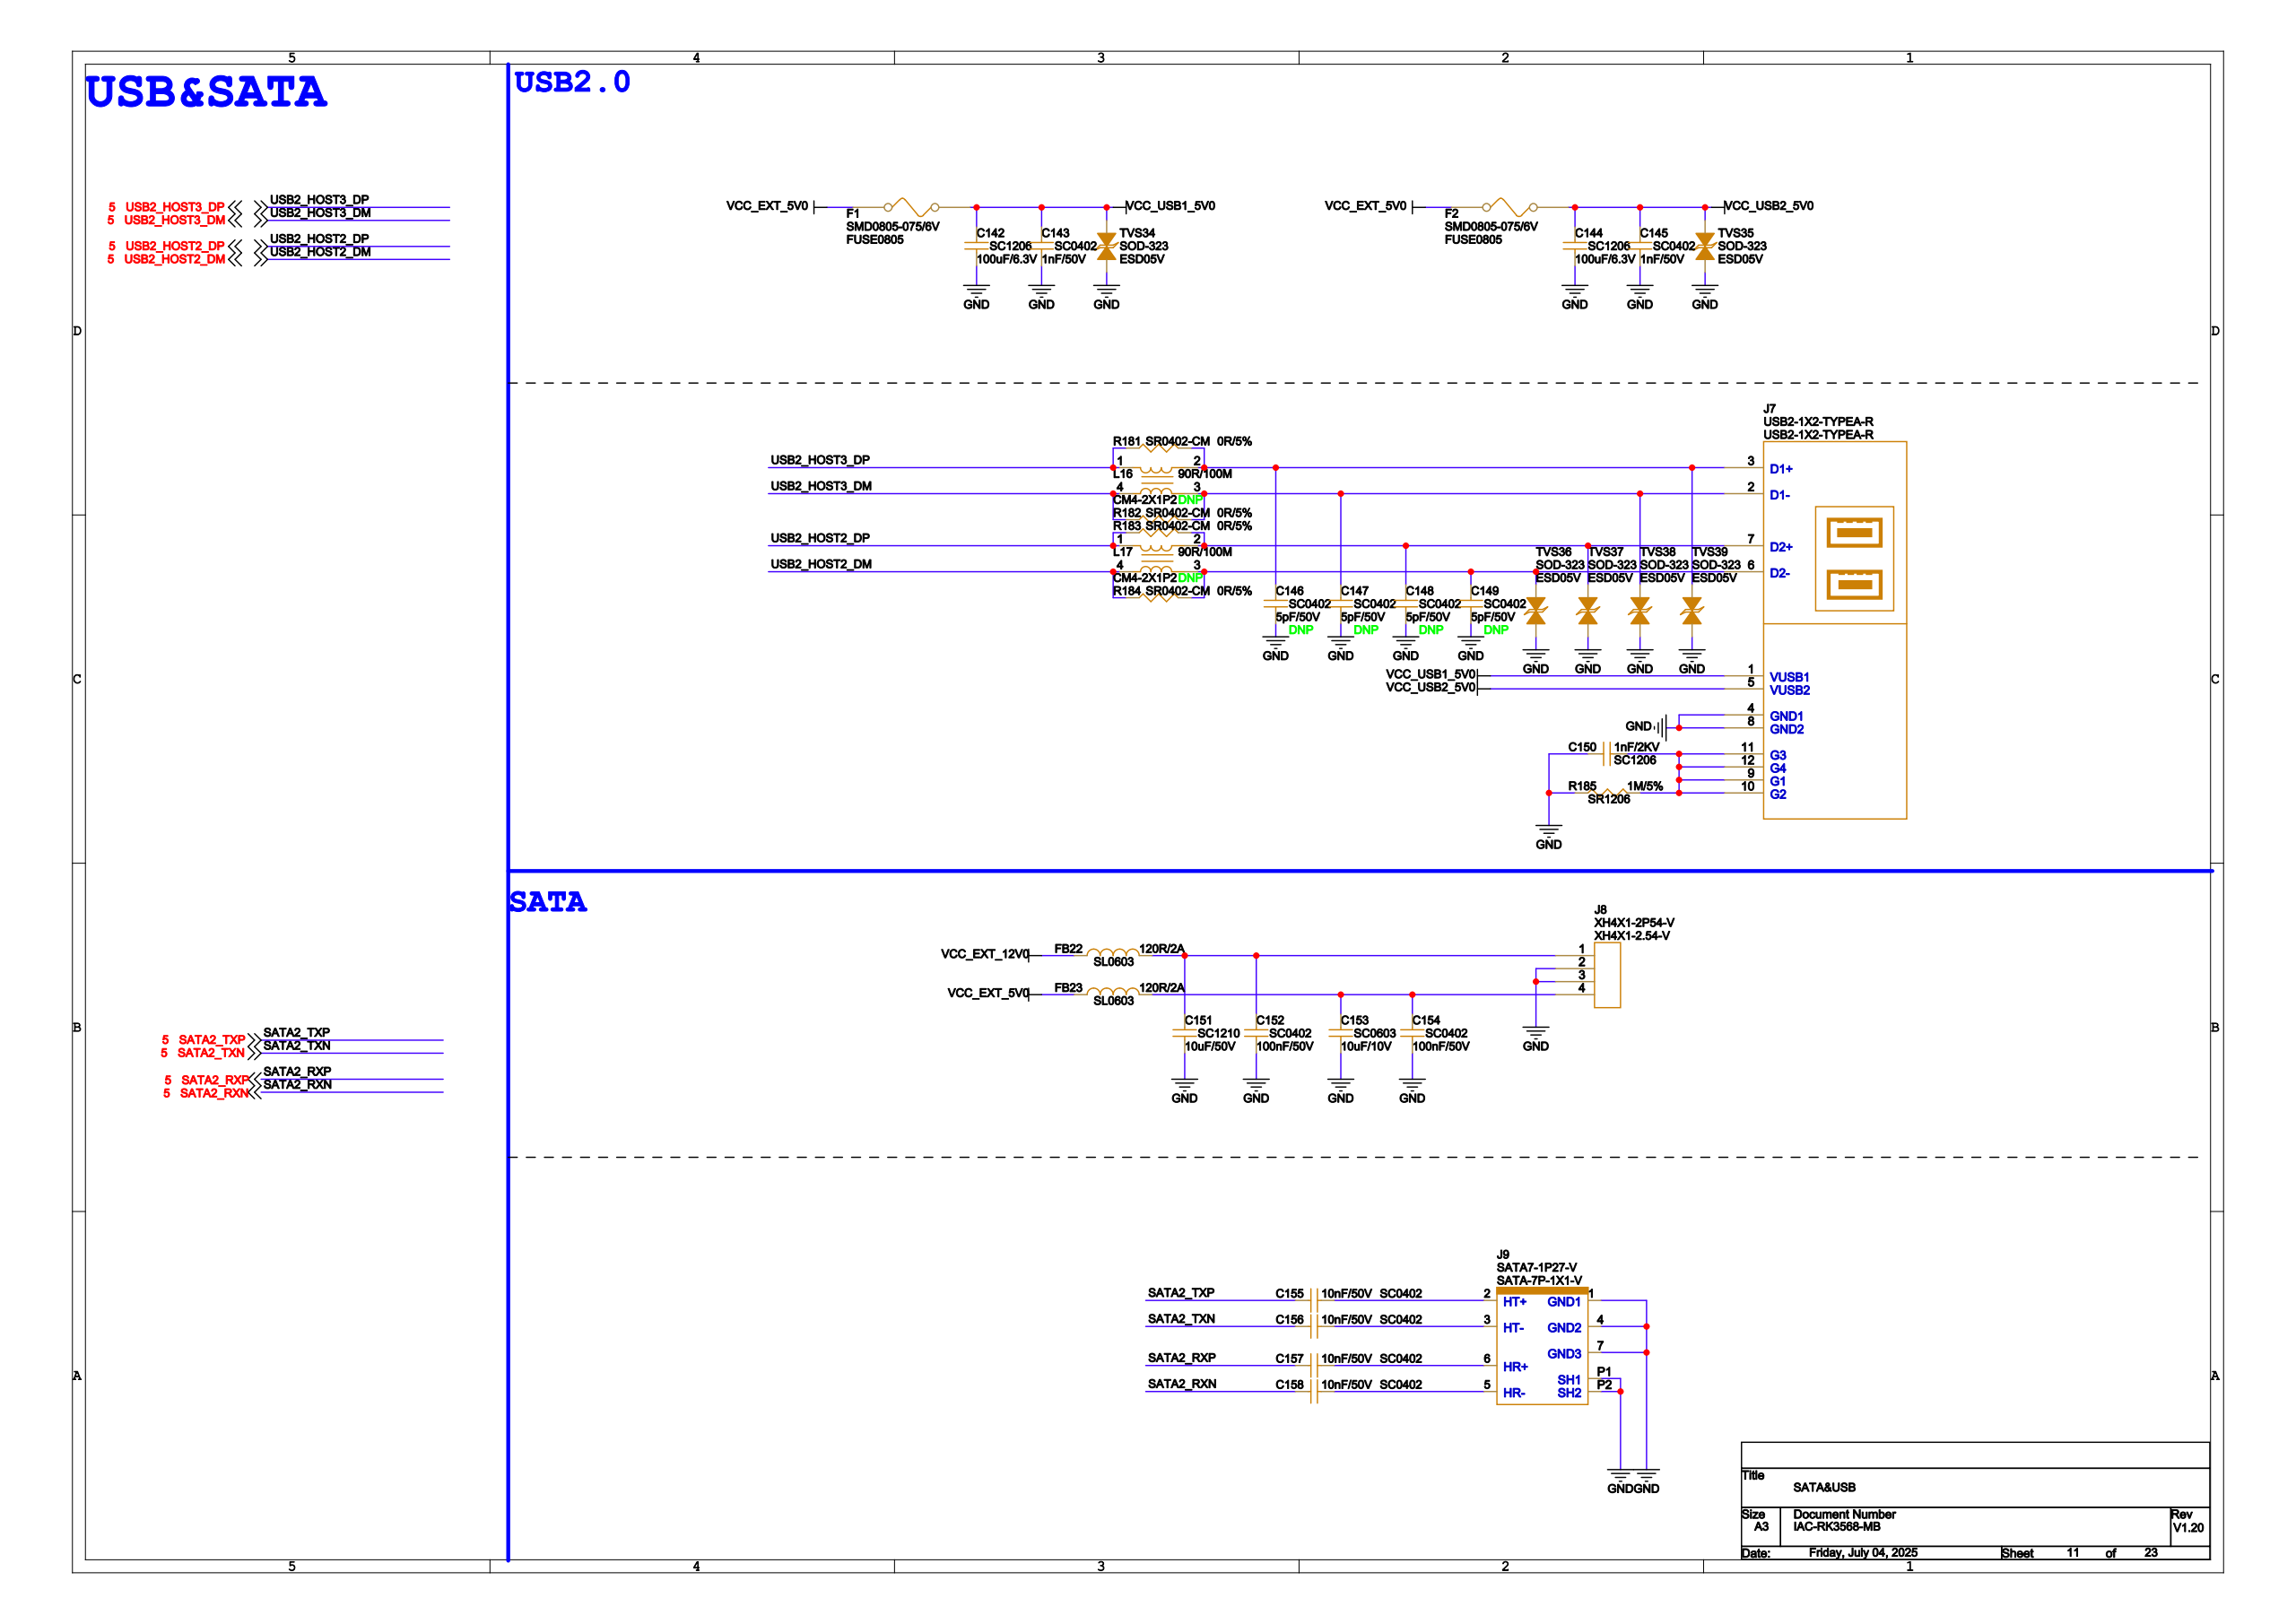Circuit board | Cadence Allegro | 1138 parts | 722 nets | one sheet of the schematic
Parts on this sheet (reference | value | footprint):
C142 | 100uF/6.3V | SC1206
C143 | 1nF/50V | SC0402
C144 | 100uF/6.3V | SC1206
C145 | 1nF/50V | SC0402
C146 | 5pF/50V | SC0402
C147 | 5pF/50V | SC0402
C148 | 5pF/50V | SC0402
C149 | 5pF/50V | SC0402
C150 | 1nF/2KV | SC1206
C151 | 10uF/50V | SC1210
C152 | 100nF/50V | SC0402
C153 | 10uF/10V | SC0603
C154 | 100nF/50V | SC0402
C155 | 10nF/50V | SC0402
C156 | 10nF/50V | SC0402
C157 | 10nF/50V | SC0402
C158 | 10nF/50V | SC0402
F1 | SMD0805-075/6V | FUSE0805
F2 | SMD0805-075/6V | FUSE0805
FB22 | 120R/2A | SL0603
FB23 | 120R/2A | SL0603
J7 | USB2-1X2-TYPEA-R | USB2-1X2-TYPEA-R
J8 | XH4X1-2.54-V | XH4X1-2P54-V
J9 | SATA-7P-1X1-V | SATA7-1P27-V
L16 | 90R/100M | CM4-2X1P2
L17 | 90R/100M | CM4-2X1P2
R181 | 0R/5% | SR0402-CM
R182 | 0R/5% | SR0402-CM
R183 | 0R/5% | SR0402-CM
R184 | 0R/5% | SR0402-CM
R185 | 1M/5% | SR1206
TVS34 | ESD05V | SOD-323
TVS35 | ESD05V | SOD-323
TVS36 | ESD05V | SOD-323
TVS37 | ESD05V | SOD-323
TVS38 | ESD05V | SOD-323
TVS39 | ESD05V | SOD-323
Nets of these parts (net: part-pin ...):
VCC_EXT_5V0: F1-2 F2-2 FB23-1
GND: C142-2 C143-2 C144-2 C145-2 C146-2 C147-2 C148-2 C149-2 C150-1 C151-2 C152-2 C153-2 C154-2 J7-4 J7-8 J8-2 J8-3 J9-1 J9-4 J9-7 J9-P1 J9-P2 R185-1 TVS34-2 TVS35-2 TVS36-1 TVS37-1 TVS38-1 TVS39-1
VCC_USB1_5V0: C142-1 C143-1 F1-1 J7-1 TVS34-1
VCC_USB2_5V0: C144-1 C145-1 F2-1 J7-5 TVS35-1
N3708542: C149-1 J7-6 L17-3 R184-2 TVS36-2
N3708514: C148-1 J7-7 L17-2 R183-2 TVS37-2
N3708486: C147-1 J7-2 L16-3 R182-2 TVS38-2
N3708458: C146-1 J7-3 L16-2 R181-2 TVS39-2
USB2_HOST3_DP: L16-1 R181-1
USB2_HOST3_DM: L16-4 R182-1
USB2_HOST2_DP: L17-1 R183-1
USB2_HOST2_DM: L17-4 R184-1
N4056971: C151-1 C152-1 FB22-2 J8-1
N4057083: C153-1 C154-1 FB23-2 J8-4
N3708818: C150-2 J7-9 J7-10 J7-11 J7-12 R185-2
SATA2_TXP: C155-1
N4056685: C155-2 J9-2
SATA2_TXN: C156-1
N4056715: C156-2 J9-3
SATA2_RXP: C157-1
N4056767: C157-2 J9-6
SATA2_RXN: C158-1
N4056771: C158-2 J9-5
VCC_EXT_12V0: FB22-1